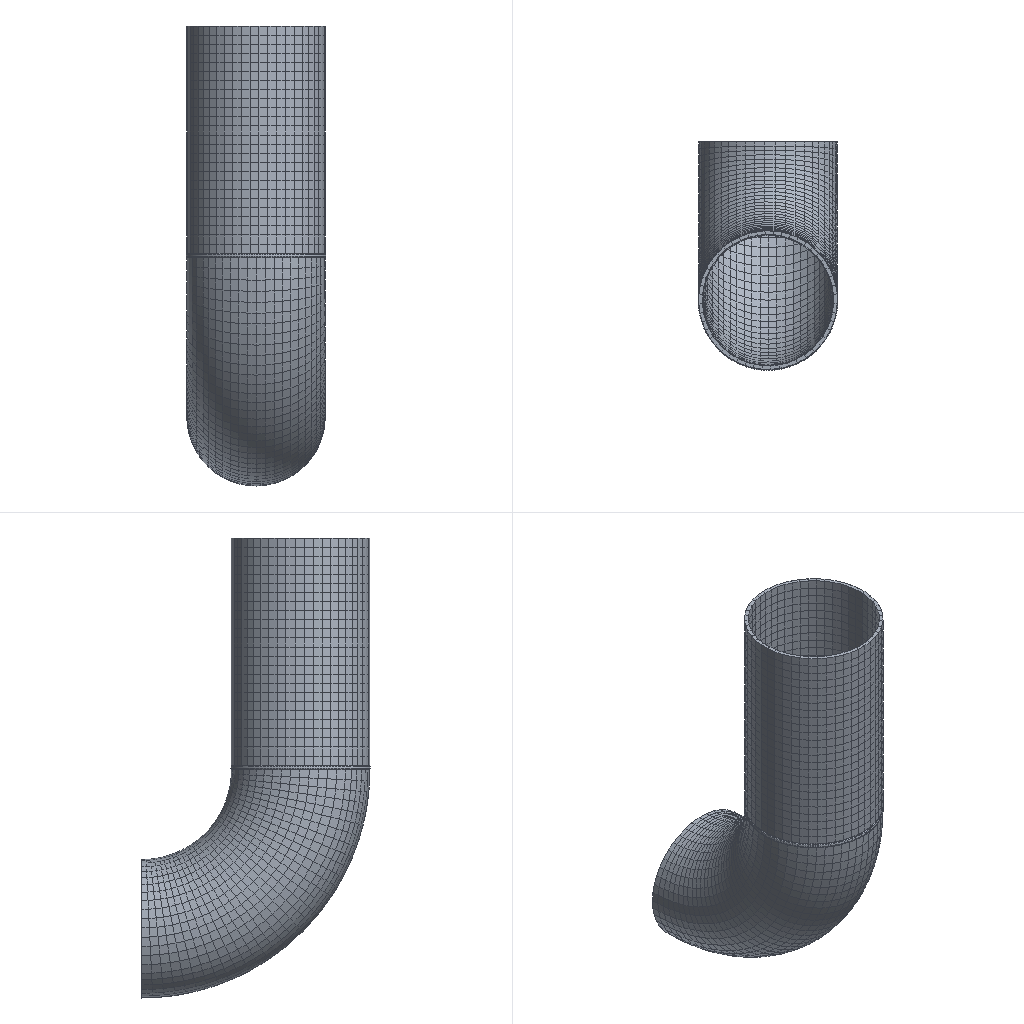Simulation study | abaqus
Set-up summary:
category,name,step,type,value,unit,region
solver,abaqus
solver,version,,,Abaqus/Standard 2020
units,not stated in the deck,,not stated
analysis,deck,,static,static
load_step,Step-1,Step-1,static
load_step,requested,,,1
mesh,nodes,,,9822
mesh,elements,,,5080
element_type,C3D8R,,solid,5080
load,load commands in deck,,count,3
bc,support commands in deck,,count,1
material,GUAN,,in results
material,HAN,,in results
check,setup vs results,,match,"per instance, exact: element labels, types and connectivity; labels of the nodes the elements use; coordinates of those nodes at SINGLE_PRECISION in 1 of 3 instance(s)"
Abaqus input file, long lists of numbers shortened:
*Heading
** Job name: Job-1 Model name: Model-1
** Generated by: Abaqus/CAE 2020
*Preprint, echo=NO, model=NO, history=NO, contact=NO
**
** PARTS
**
*Part, name=crack
*End Part
**
*Part, name=hanfeng
*Node
      1,   285.9,         -75.,           0.
      2,    292.646,         -75.,           0.
** (4222 more lines like these left out)
*Element, type=C3D8R
   1,   17,   18,   22,   21,    1,    2,    6,    5
   2,   18,   19,   23,   22,    2,    3,    7,    6
** (2374 more lines like these left out)
*Nset, nset=Set-2, generate
    1,  4224,     1
*Elset, elset=Set-2, generate
    1,  2376,     1
** Section: han
*Solid Section, elset=Set-2, material=han
,
*End Part
**
*Part, name=wantou
*Node
      1,           0.,  -400.863,  -59.514
      2,           0.,  -419.684,  -56.228
** (3100 more lines like these left out)
*Element, type=C3D8R
   1,   95,   96,  106,  115,    1,    2,   12,   21
   2,  115,  106,  107,  114,   21,   12,   13,   20
** (1502 more lines like these left out)
*Nset, nset=Set-2, generate
    1,  3102,     1
*Elset, elset=Set-2, generate
    1,  1504,     1
** Section: guan
*Solid Section, elset=Set-2, material=guan
,
*End Part
**
*Part, name=zhiguan
*Node
      1,   234.565,   168.991,           0.
      2,   247.669,   178.003,           0.
** (2494 more lines like these left out)
*Element, type=C3D8R
   1,   97,   98,  106,  128,    1,    2,   10,   32
   2,  128,  106,  107,  127,   32,   10,   11,   31
** (1198 more lines like these left out)
*Nset, nset=Set-2, generate
    1,  2496,     1
*Elset, elset=Set-2, generate
    1,  1200,     1
** Section: guan
*Solid Section, elset=Set-2, material=guan
,
*End Part
**
**
** ASSEMBLY
**
*Assembly, name=Assembly
**
*Instance, name=wantou-1, part=wantou
          0.,         700.,           0.
          0.,         700.,           0.,           0., 701.,           0., 90.
*End Instance
**
*Instance, name=zhiguan-1, part=zhiguan
          0.,           0.,          20.
*End Instance
**
*Instance, name=hanfeng-1, part=hanfeng
          0.,           0.,          75.
          0.,           0.,          75., 1.,           0.,          75., 90.
*End Instance
**
*Instance, name=crack-1, part=crack
   302.153,           0.,    10.6
*End Instance
**
*Node
      1,           0., -1.86758635e-14,        1020.
*Nset, nset=Set-3, instance=wantou-1, generate
 3009,  3102,     1
*Elset, elset=Set-3, instance=wantou-1, generate
 1458,  1504,     1
*Nset, nset=Set-5
 1,
*Nset, nset=Set-6
 1,
*Nset, nset=m_Set-4
 1,
*Nset, nset=_PickedSet14, internal, instance=hanfeng-1, generate
    1,  4224,     1
*Elset, elset=_PickedSet14, internal, instance=hanfeng-1, generate
    1,  2376,     1
*Elset, elset=_Surf-5_S4, internal, instance=wantou-1
    1,    2,    3,    4,    5,    6,   31,   32,   33,   34,   35,   36,   48,   49,   50,   51
   52,   53,   78,   79,   80,   81,   82,   83,   95,   96,   97,   98,   99,  100,  125,  126
** (22 more lines like these left out)
*Elset, elset=_Surf-5_S4, internal, instance=zhiguan-1
   14,   15,   16,   17,   18,   19,   20,   21,   22,   23,   24,   25,   26,   27,   28,   29
   30,   31,   32,   33,   62,   63,   64,   65,   66,   67,   68,   69,   70,   71,   72,   73
** (30 more lines like these left out)
*Elset, elset=_Surf-5_S6, internal, instance=wantou-1
    7,    8,    9,   10,   11,   12,   13,   14,   15,   16,   17,   18,   19,   20,   21,   22
   23,   24,   25,   26,   27,   28,   29,   30,   37,   38,   39,   40,   41,   42,   43,   44
** (68 more lines like these left out)
*Elset, elset=_Surf-5_S6, internal, instance=zhiguan-1
    1,    2,    3,    4,    5,    6,    7,    8,    9,   10,   11,   12,   13,   34,   35,   36
   37,   38,   39,   40,   41,   42,   43,   44,   45,   46,   47,   48,   49,   50,   51,   52
** (42 more lines like these left out)
*Surface, type=ELEMENT, name=Surf-5
_Surf-5_S4, S4
_Surf-5_S6, S6
*Elset, elset=_m_Surf-1_S2, internal, instance=zhiguan-1, generate
  1,  48,   1
*Surface, type=ELEMENT, name=m_Surf-1
_m_Surf-1_S2, S2
*Elset, elset=_m_Surf-3_S2, internal, instance=wantou-1, generate
  1,  47,   1
*Surface, type=ELEMENT, name=m_Surf-3
_m_Surf-3_S2, S2
*Elset, elset=_s_Surf-1_S5, internal, instance=hanfeng-1
    7,    8,    9,   16,   17,   18,   25,   26,   27,   34,   35,   36,   43,   44,   45,   52
   53,   54,   61,   62,   63,   70,   71,   72,   79,   80,   81,   88,   89,   90,   97,   98
** (48 more lines like these left out)
*Surface, type=ELEMENT, name=s_Surf-1
_s_Surf-1_S5, S5
*Elset, elset=_s_Surf-3_S3, internal, instance=hanfeng-1
    1,    2,    3,   10,   11,   12,   19,   20,   21,   28,   29,   30,   37,   38,   39,   46
   47,   48,   55,   56,   57,   64,   65,   66,   73,   74,   75,   82,   83,   84,   91,   92
** (48 more lines like these left out)
*Surface, type=ELEMENT, name=s_Surf-3
_s_Surf-3_S3, S3
*Elset, elset=_s_Surf-6_S1, internal, instance=zhiguan-1, generate
 1153,  1200,     1
*Surface, type=ELEMENT, name=s_Surf-6
_s_Surf-6_S1, S1
** Constraint: Constraint-1
*Tie, name=Constraint-1, adjust=yes
s_Surf-1, m_Surf-1
** Constraint: Constraint-2
*Tie, name=Constraint-2, adjust=yes
s_Surf-3, m_Surf-3
** Constraint: Constraint-3
*Coupling, constraint name=Constraint-3, ref node=m_Set-4, surface=s_Surf-6
*Kinematic
*Enrichment, name=Crack-1, type=PROPAGATION CRACK, elset=_PickedSet14
*End Assembly
*Amplitude, name=Amp-1
             0.,              0.,              1.,              1.
**
** MATERIALS
**
*Material, name=guan
*Elastic
210000., 0.3
*Plastic
406.,0.
*Material, name=han
*Damage Initiation, criterion=QUADE
 5e-05, 5e-05, 5e-05
*Damage Evolution, type=DISPLACEMENT
 1e-06,
*Elastic
180000., 0.3
*Initial Conditions, type=ENRICHMENT
hanfeng-1.236, 1,Crack-1, -3.696, 2.403
hanfeng-1.236, 2,Crack-1, -3.643, -2.571
hanfeng-1.236, 3,Crack-1, 4.53, -1.547
hanfeng-1.236, 4,Crack-1, 3.288, 2.843
hanfeng-1.236, 5,Crack-1, -3.696, 7.972
hanfeng-1.236, 6,Crack-1, -3.643, 3.144
hanfeng-1.236, 7,Crack-1, 4.53, 4.138
hanfeng-1.236, 8,Crack-1, 3.288, 8.399
hanfeng-1.237, 1,Crack-1, -3.696, 6.445
hanfeng-1.237, 2,Crack-1, -3.643, -0.6509
hanfeng-1.237, 3,Crack-1, 4.53, 0.8094
hanfeng-1.237, 4,Crack-1, 3.288, 7.073
hanfeng-1.237, 5,Crack-1, -3.696, 2.403
hanfeng-1.237, 6,Crack-1, -3.643, -2.571
hanfeng-1.237, 7,Crack-1, 4.53, -1.547
hanfeng-1.237, 8,Crack-1, 3.288, 2.843
** ----------------------------------------------------------------
**
** STEP: Step-1
**
*Step, name=Step-1, nlgeom=YES, inc=1000
*Static, stabilize=0.0002, allsdtol=0.05, continue=NO
0.01, 1., 1e-07, 1.
**
** BOUNDARY CONDITIONS
**
** Name: BC-1 Type: 对称/反对称/完全固定
*Boundary
Set-3, ENCASTRE
**
** LOADS
**
** Name: Load-1   Type: Pressure
*Dsload, amplitude=Amp-1
Surf-5, P, 0.05
** Name: Load-3   Type: Concentrated force
*Cload, amplitude=Amp-1
Set-6, 3, 10000.
** Name: Load-y   Type: Concentrated force
*Cload, amplitude=Amp-1
Set-5, 2, 50000.
**
** CONTROLS
**
*Controls, reset
*Controls, parameters=time incrementation
, , , , , , , 20, , ,
**
** OUTPUT REQUESTS
**
*Restart, write, frequency=0
**
** FIELD OUTPUT: F-Output-1
**
*Output, field
*Node Output
CF, PHILSM, PSILSM, RF, RM, RT, TF, U
V
*Element Output, directions=YES
E, ENRRTXFEM, LE, LOADSXFEM, MISES, MISESMAX, MISESONLY, PE, PEEQ, PEMAG, S, SDEG, SF, SSAVG, STATUS, STATUSXFEM
*Contact Output
CDISP, CSTRESS
**
** HISTORY OUTPUT: H-Output-1
**
*Output, history, variable=PRESELECT
*End Step
Results summary:
result,step,,partial,increments=22 time=0.3556/1.0
result,analysis,,,static
result,last_loadstep,,,1
result,primary field,,,U
result,reaction total,,FX,1.234,model units
result,reaction total,,FY,-13212.341,model units
result,reaction total,,FZ,997.587,model units